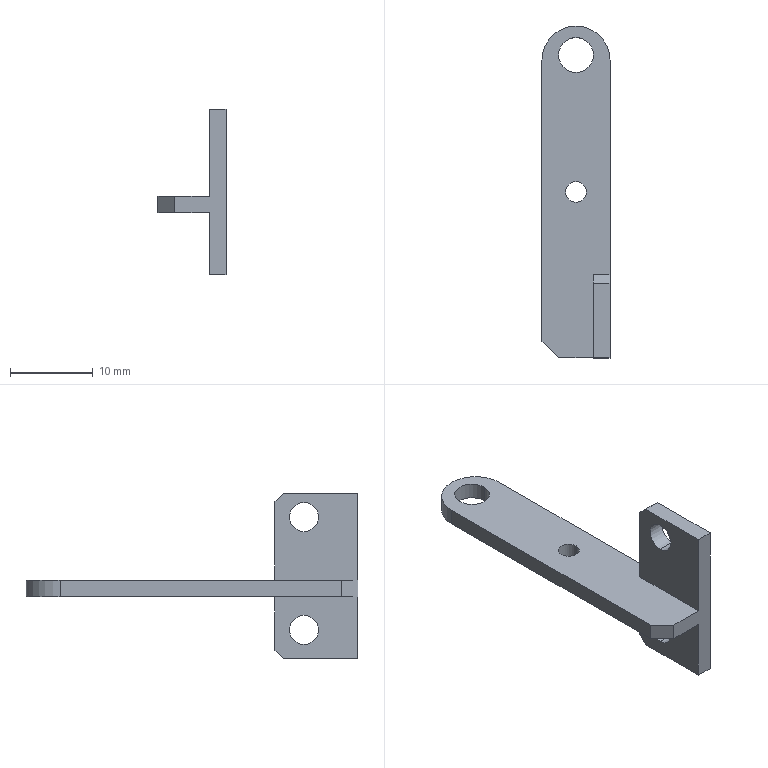Part | STEP file | 11-FG-B07711 | 1 solid | 24 faces | box 8.2 x 40 x 20 mm | volume 919.559 mm3 | plane 14 | cylinder 10 | commonest cylinder face diameters 3.5 x4 2.5 x2 4.2 x2 8.2 x2
STEP:
#1=CARTESIAN_POINT('',(-1.25,0.,0.));
#2=VERTEX_POINT('',#1);
#3=CARTESIAN_POINT('',(1.25,0.,0.));
#4=VERTEX_POINT('',#3);
#5=CARTESIAN_POINT('',(0.,0.,0.));
#6=DIRECTION('',(0.,0.,1.));
#7=DIRECTION('',(1.,0.,0.));
#8=AXIS2_PLACEMENT_3D('',#5,#6,#7);
#9=CIRCLE('',#8,1.25);
#10=EDGE_CURVE('',#2,#4,#9,.T.);
#11=ORIENTED_EDGE('',*,*,#10,.F.);
#12=CARTESIAN_POINT('',(-1.25,0.,2.));
#13=VERTEX_POINT('',#12);
#14=CARTESIAN_POINT('',(-1.25,0.,2.));
#15=DIRECTION('',(0.,0.,1.));
#16=VECTOR('',#15,1000.);
#17=LINE('',#14,#16);
#18=EDGE_CURVE('',#2,#13,#17,.T.);
#19=ORIENTED_EDGE('',*,*,#18,.T.);
#20=CARTESIAN_POINT('',(1.25,0.,2.));
#21=VERTEX_POINT('',#20);
#22=CARTESIAN_POINT('',(0.,0.,2.));
#23=DIRECTION('',(0.,0.,1.));
#24=DIRECTION('',(1.,0.,0.));
#25=AXIS2_PLACEMENT_3D('',#22,#23,#24);
#26=CIRCLE('',#25,1.25);
#27=EDGE_CURVE('',#13,#21,#26,.T.);
#28=ORIENTED_EDGE('',*,*,#27,.T.);
#29=CARTESIAN_POINT('',(1.25,0.,2.));
#30=DIRECTION('',(0.,0.,1.));
#31=VECTOR('',#30,1000.);
#32=LINE('',#29,#31);
#33=EDGE_CURVE('',#4,#21,#32,.T.);
#34=ORIENTED_EDGE('',*,*,#33,.F.);
#35=EDGE_LOOP('',(#11,#19,#28,#34));
#36=FACE_OUTER_BOUND('',#35,.T.);
#37=CARTESIAN_POINT('',(0.,0.,2.));
#38=DIRECTION('',(0.,0.,1.));
#39=DIRECTION('',(1.,0.,0.));
#40=AXIS2_PLACEMENT_3D('',#37,#38,#39);
#41=CYLINDRICAL_SURFACE('',#40,1.25);
#42=ADVANCED_FACE('',(#36),#41,.F.);
#43=CARTESIAN_POINT('',(4.1,-13.5,-5.75));
#44=VERTEX_POINT('',#43);
#45=CARTESIAN_POINT('',(4.1,-13.5,-2.25));
#46=VERTEX_POINT('',#45);
#47=CARTESIAN_POINT('',(4.1,-13.5,-4.));
#48=DIRECTION('',(-1.,0.,0.));
#49=DIRECTION('',(0.,-1.,0.));
#50=AXIS2_PLACEMENT_3D('',#47,#48,#49);
#51=CIRCLE('',#50,1.75);
#52=EDGE_CURVE('',#44,#46,#51,.T.);
#53=ORIENTED_EDGE('',*,*,#52,.F.);
#54=CARTESIAN_POINT('',(2.1,-13.5,-5.75));
#55=VERTEX_POINT('',#54);
#56=CARTESIAN_POINT('',(9.6,-13.5,-5.75));
#57=DIRECTION('',(-1.,0.,0.));
#58=VECTOR('',#57,1000.);
#59=LINE('',#56,#58);
#60=EDGE_CURVE('',#44,#55,#59,.T.);
#61=ORIENTED_EDGE('',*,*,#60,.T.);
#62=CARTESIAN_POINT('',(2.1,-13.5,-2.25));
#63=VERTEX_POINT('',#62);
#64=CARTESIAN_POINT('',(2.1,-13.5,-4.));
#65=DIRECTION('',(-1.,0.,0.));
#66=DIRECTION('',(0.,0.,1.));
#67=AXIS2_PLACEMENT_3D('',#64,#65,#66);
#68=CIRCLE('',#67,1.75);
#69=EDGE_CURVE('',#55,#63,#68,.T.);
#70=ORIENTED_EDGE('',*,*,#69,.T.);
#71=CARTESIAN_POINT('',(9.6,-13.5,-2.25));
#72=DIRECTION('',(-1.,0.,0.));
#73=VECTOR('',#72,1000.);
#74=LINE('',#71,#73);
#75=EDGE_CURVE('',#46,#63,#74,.T.);
#76=ORIENTED_EDGE('',*,*,#75,.F.);
#77=EDGE_LOOP('',(#53,#61,#70,#76));
#78=FACE_OUTER_BOUND('',#77,.T.);
#79=CARTESIAN_POINT('',(9.6,-13.5,-4.));
#80=DIRECTION('',(-1.,0.,0.));
#81=DIRECTION('',(0.,0.,1.));
#82=AXIS2_PLACEMENT_3D('',#79,#80,#81);
#83=CYLINDRICAL_SURFACE('',#82,1.75);
#84=ADVANCED_FACE('',(#78),#83,.F.);
#85=CARTESIAN_POINT('',(4.1,-13.5,7.85));
#86=VERTEX_POINT('',#85);
#87=CARTESIAN_POINT('',(4.1,-13.5,11.35));
#88=VERTEX_POINT('',#87);
#89=CARTESIAN_POINT('',(4.1,-13.5,9.6));
#90=DIRECTION('',(-1.,0.,0.));
#91=DIRECTION('',(0.,-1.,0.));
#92=AXIS2_PLACEMENT_3D('',#89,#90,#91);
#93=CIRCLE('',#92,1.75);
#94=EDGE_CURVE('',#86,#88,#93,.T.);
#95=ORIENTED_EDGE('',*,*,#94,.F.);
#96=CARTESIAN_POINT('',(2.1,-13.5,7.85));
#97=VERTEX_POINT('',#96);
#98=CARTESIAN_POINT('',(9.6,-13.5,7.85));
#99=DIRECTION('',(-1.,0.,0.));
#100=VECTOR('',#99,1000.);
#101=LINE('',#98,#100);
#102=EDGE_CURVE('',#86,#97,#101,.T.);
#103=ORIENTED_EDGE('',*,*,#102,.T.);
#104=CARTESIAN_POINT('',(2.1,-13.5,11.35));
#105=VERTEX_POINT('',#104);
#106=CARTESIAN_POINT('',(2.1,-13.5,9.6));
#107=DIRECTION('',(-1.,0.,0.));
#108=DIRECTION('',(0.,0.,1.));
#109=AXIS2_PLACEMENT_3D('',#106,#107,#108);
#110=CIRCLE('',#109,1.75);
#111=EDGE_CURVE('',#97,#105,#110,.T.);
#112=ORIENTED_EDGE('',*,*,#111,.T.);
#113=CARTESIAN_POINT('',(9.6,-13.5,11.35));
#114=DIRECTION('',(-1.,0.,0.));
#115=VECTOR('',#114,1000.);
#116=LINE('',#113,#115);
#117=EDGE_CURVE('',#88,#105,#116,.T.);
#118=ORIENTED_EDGE('',*,*,#117,.F.);
#119=EDGE_LOOP('',(#95,#103,#112,#118));
#120=FACE_OUTER_BOUND('',#119,.T.);
#121=CARTESIAN_POINT('',(9.6,-13.5,9.6));
#122=DIRECTION('',(-1.,0.,0.));
#123=DIRECTION('',(0.,0.,1.));
#124=AXIS2_PLACEMENT_3D('',#121,#122,#123);
#125=CYLINDRICAL_SURFACE('',#124,1.75);
#126=ADVANCED_FACE('',(#120),#125,.F.);
#127=CARTESIAN_POINT('',(-2.1,16.5,0.));
#128=VERTEX_POINT('',#127);
#129=CARTESIAN_POINT('',(2.1,16.5,0.));
#130=VERTEX_POINT('',#129);
#131=CARTESIAN_POINT('',(0.,16.5,0.));
#132=DIRECTION('',(0.,0.,1.));
#133=DIRECTION('',(1.,0.,0.));
#134=AXIS2_PLACEMENT_3D('',#131,#132,#133);
#135=CIRCLE('',#134,2.1);
#136=EDGE_CURVE('',#128,#130,#135,.T.);
#137=ORIENTED_EDGE('',*,*,#136,.F.);
#138=CARTESIAN_POINT('',(-2.1,16.5,2.));
#139=VERTEX_POINT('',#138);
#140=CARTESIAN_POINT('',(-2.1,16.5,0.));
#141=DIRECTION('',(0.,0.,1.));
#142=VECTOR('',#141,1000.);
#143=LINE('',#140,#142);
#144=EDGE_CURVE('',#128,#139,#143,.T.);
#145=ORIENTED_EDGE('',*,*,#144,.T.);
#146=CARTESIAN_POINT('',(2.1,16.5,2.));
#147=VERTEX_POINT('',#146);
#148=CARTESIAN_POINT('',(0.,16.5,2.));
#149=DIRECTION('',(0.,0.,1.));
#150=DIRECTION('',(1.,0.,0.));
#151=AXIS2_PLACEMENT_3D('',#148,#149,#150);
#152=CIRCLE('',#151,2.1);
#153=EDGE_CURVE('',#139,#147,#152,.T.);
#154=ORIENTED_EDGE('',*,*,#153,.T.);
#155=CARTESIAN_POINT('',(2.1,16.5,0.));
#156=DIRECTION('',(0.,0.,1.));
#157=VECTOR('',#156,1000.);
#158=LINE('',#155,#157);
#159=EDGE_CURVE('',#130,#147,#158,.T.);
#160=ORIENTED_EDGE('',*,*,#159,.F.);
#161=EDGE_LOOP('',(#137,#145,#154,#160));
#162=FACE_OUTER_BOUND('',#161,.T.);
#163=CARTESIAN_POINT('',(0.,16.5,0.));
#164=DIRECTION('',(0.,0.,1.));
#165=DIRECTION('',(1.,0.,0.));
#166=AXIS2_PLACEMENT_3D('',#163,#164,#165);
#167=CYLINDRICAL_SURFACE('',#166,2.1);
#168=ADVANCED_FACE('',(#162),#167,.F.);
#169=CARTESIAN_POINT('',(0.,0.,0.));
#170=DIRECTION('',(0.,0.,1.));
#171=DIRECTION('',(1.,0.,0.));
#172=AXIS2_PLACEMENT_3D('',#169,#170,#171);
#173=CIRCLE('',#172,1.25);
#174=EDGE_CURVE('',#4,#2,#173,.T.);
#175=ORIENTED_EDGE('',*,*,#174,.T.);
#176=ORIENTED_EDGE('',*,*,#10,.T.);
#177=EDGE_LOOP('',(#175,#176));
#178=FACE_BOUND('',#177,.T.);
#179=CARTESIAN_POINT('',(0.,16.5,0.));
#180=DIRECTION('',(0.,0.,1.));
#181=DIRECTION('',(1.,0.,0.));
#182=AXIS2_PLACEMENT_3D('',#179,#180,#181);
#183=CIRCLE('',#182,2.1);
#184=EDGE_CURVE('',#130,#128,#183,.T.);
#185=ORIENTED_EDGE('',*,*,#184,.T.);
#186=ORIENTED_EDGE('',*,*,#136,.T.);
#187=EDGE_LOOP('',(#185,#186));
#188=FACE_BOUND('',#187,.T.);
#189=CARTESIAN_POINT('',(-2.1,-20.,0.));
#190=VERTEX_POINT('',#189);
#191=CARTESIAN_POINT('',(2.1,-20.,0.));
#192=VERTEX_POINT('',#191);
#193=CARTESIAN_POINT('',(-14.1,-20.,0.));
#194=DIRECTION('',(1.,0.,0.));
#195=VECTOR('',#194,1000.);
#196=LINE('',#193,#195);
#197=EDGE_CURVE('',#190,#192,#196,.T.);
#198=ORIENTED_EDGE('',*,*,#197,.F.);
#199=CARTESIAN_POINT('',(-4.1,-18.,0.));
#200=VERTEX_POINT('',#199);
#201=CARTESIAN_POINT('',(-4.1,-18.,0.));
#202=DIRECTION('',(-0.7071,0.7071,0.));
#203=VECTOR('',#202,1000.);
#204=LINE('',#201,#203);
#205=EDGE_CURVE('',#190,#200,#204,.T.);
#206=ORIENTED_EDGE('',*,*,#205,.T.);
#207=CARTESIAN_POINT('',(-4.1,15.9,0.));
#208=VERTEX_POINT('',#207);
#209=CARTESIAN_POINT('',(-4.1,20.,0.));
#210=DIRECTION('',(0.,1.,0.));
#211=VECTOR('',#210,1000.);
#212=LINE('',#209,#211);
#213=EDGE_CURVE('',#200,#208,#212,.T.);
#214=ORIENTED_EDGE('',*,*,#213,.T.);
#215=CARTESIAN_POINT('',(0.,20.,0.));
#216=VERTEX_POINT('',#215);
#217=CARTESIAN_POINT('',(0.,15.9,0.));
#218=DIRECTION('',(0.,0.,-1.));
#219=DIRECTION('',(1.,0.,0.));
#220=AXIS2_PLACEMENT_3D('',#217,#218,#219);
#221=CIRCLE('',#220,4.1);
#222=EDGE_CURVE('',#208,#216,#221,.T.);
#223=ORIENTED_EDGE('',*,*,#222,.T.);
#224=CARTESIAN_POINT('',(4.1,15.9,0.));
#225=VERTEX_POINT('',#224);
#226=CARTESIAN_POINT('',(0.,15.9,0.));
#227=DIRECTION('',(0.,0.,-1.));
#228=DIRECTION('',(1.,0.,0.));
#229=AXIS2_PLACEMENT_3D('',#226,#227,#228);
#230=CIRCLE('',#229,4.1);
#231=EDGE_CURVE('',#216,#225,#230,.T.);
#232=ORIENTED_EDGE('',*,*,#231,.T.);
#233=CARTESIAN_POINT('',(4.1,-10.,0.));
#234=VERTEX_POINT('',#233);
#235=CARTESIAN_POINT('',(4.1,20.,0.));
#236=DIRECTION('',(0.,-1.,0.));
#237=VECTOR('',#236,1000.);
#238=LINE('',#235,#237);
#239=EDGE_CURVE('',#225,#234,#238,.T.);
#240=ORIENTED_EDGE('',*,*,#239,.T.);
#241=CARTESIAN_POINT('',(2.1,-10.,0.));
#242=VERTEX_POINT('',#241);
#243=CARTESIAN_POINT('',(2.1,-10.,0.));
#244=DIRECTION('',(1.,0.,0.));
#245=VECTOR('',#244,1000.);
#246=LINE('',#243,#245);
#247=EDGE_CURVE('',#242,#234,#246,.T.);
#248=ORIENTED_EDGE('',*,*,#247,.F.);
#249=CARTESIAN_POINT('',(2.1,-10.,0.));
#250=DIRECTION('',(0.,1.,0.));
#251=VECTOR('',#250,1000.);
#252=LINE('',#249,#251);
#253=EDGE_CURVE('',#192,#242,#252,.T.);
#254=ORIENTED_EDGE('',*,*,#253,.F.);
#255=EDGE_LOOP('',(#198,#206,#214,#223,#232,#240,#248,#254));
#256=FACE_OUTER_BOUND('',#255,.T.);
#257=CARTESIAN_POINT('',(0.,0.,0.));
#258=DIRECTION('',(0.,0.,1.));
#259=DIRECTION('',(1.,0.,0.));
#260=AXIS2_PLACEMENT_3D('',#257,#258,#259);
#261=PLANE('',#260);
#262=ADVANCED_FACE('',(#178,#188,#256),#261,.F.);
#263=CARTESIAN_POINT('',(-2.1,-20.,2.));
#264=VERTEX_POINT('',#263);
#265=CARTESIAN_POINT('',(2.1,-20.,2.));
#266=VERTEX_POINT('',#265);
#267=CARTESIAN_POINT('',(-14.1,-20.,2.));
#268=DIRECTION('',(1.,0.,0.));
#269=VECTOR('',#268,1000.);
#270=LINE('',#267,#269);
#271=EDGE_CURVE('',#264,#266,#270,.T.);
#272=ORIENTED_EDGE('',*,*,#271,.F.);
#273=CARTESIAN_POINT('',(-2.1,-20.,2.));
#274=DIRECTION('',(0.,0.,-1.));
#275=VECTOR('',#274,1000.);
#276=LINE('',#273,#275);
#277=EDGE_CURVE('',#264,#190,#276,.T.);
#278=ORIENTED_EDGE('',*,*,#277,.T.);
#279=ORIENTED_EDGE('',*,*,#197,.T.);
#280=CARTESIAN_POINT('',(2.1,-20.,-7.5));
#281=VERTEX_POINT('',#280);
#282=CARTESIAN_POINT('',(2.1,-20.,-7.5));
#283=DIRECTION('',(0.,0.,1.));
#284=VECTOR('',#283,1000.);
#285=LINE('',#282,#284);
#286=EDGE_CURVE('',#281,#192,#285,.T.);
#287=ORIENTED_EDGE('',*,*,#286,.F.);
#288=CARTESIAN_POINT('',(4.1,-20.,-7.5));
#289=VERTEX_POINT('',#288);
#290=CARTESIAN_POINT('',(2.1,-20.,-7.5));
#291=DIRECTION('',(-1.,0.,0.));
#292=VECTOR('',#291,1000.);
#293=LINE('',#290,#292);
#294=EDGE_CURVE('',#289,#281,#293,.T.);
#295=ORIENTED_EDGE('',*,*,#294,.F.);
#296=CARTESIAN_POINT('',(4.1,-20.,12.5));
#297=VERTEX_POINT('',#296);
#298=CARTESIAN_POINT('',(4.1,-20.,-22.));
#299=DIRECTION('',(0.,0.,1.));
#300=VECTOR('',#299,1000.);
#301=LINE('',#298,#300);
#302=EDGE_CURVE('',#289,#297,#301,.T.);
#303=ORIENTED_EDGE('',*,*,#302,.T.);
#304=CARTESIAN_POINT('',(2.1,-20.,12.5));
#305=VERTEX_POINT('',#304);
#306=CARTESIAN_POINT('',(4.1,-20.,12.5));
#307=DIRECTION('',(1.,0.,0.));
#308=VECTOR('',#307,1000.);
#309=LINE('',#306,#308);
#310=EDGE_CURVE('',#305,#297,#309,.T.);
#311=ORIENTED_EDGE('',*,*,#310,.F.);
#312=CARTESIAN_POINT('',(2.1,-20.,12.5));
#313=DIRECTION('',(0.,0.,-1.));
#314=VECTOR('',#313,1000.);
#315=LINE('',#312,#314);
#316=EDGE_CURVE('',#305,#266,#315,.T.);
#317=ORIENTED_EDGE('',*,*,#316,.T.);
#318=EDGE_LOOP('',(#272,#278,#279,#287,#295,#303,#311,#317));
#319=FACE_OUTER_BOUND('',#318,.T.);
#320=CARTESIAN_POINT('',(-14.1,-20.,2.));
#321=DIRECTION('',(0.,1.,0.));
#322=DIRECTION('',(0.,0.,1.));
#323=AXIS2_PLACEMENT_3D('',#320,#321,#322);
#324=PLANE('',#323);
#325=ADVANCED_FACE('',(#319),#324,.F.);
#326=CARTESIAN_POINT('',(0.,0.,2.));
#327=DIRECTION('',(0.,0.,1.));
#328=DIRECTION('',(1.,0.,0.));
#329=AXIS2_PLACEMENT_3D('',#326,#327,#328);
#330=CIRCLE('',#329,1.25);
#331=EDGE_CURVE('',#21,#13,#330,.T.);
#332=ORIENTED_EDGE('',*,*,#331,.F.);
#333=ORIENTED_EDGE('',*,*,#27,.F.);
#334=EDGE_LOOP('',(#332,#333));
#335=FACE_BOUND('',#334,.T.);
#336=CARTESIAN_POINT('',(-4.1,-18.,2.));
#337=VERTEX_POINT('',#336);
#338=CARTESIAN_POINT('',(-4.1,15.9,2.));
#339=VERTEX_POINT('',#338);
#340=CARTESIAN_POINT('',(-4.1,20.,2.));
#341=DIRECTION('',(0.,1.,0.));
#342=VECTOR('',#341,1000.);
#343=LINE('',#340,#342);
#344=EDGE_CURVE('',#337,#339,#343,.T.);
#345=ORIENTED_EDGE('',*,*,#344,.F.);
#346=CARTESIAN_POINT('',(-11.05,-11.05,2.));
#347=DIRECTION('',(0.7071,-0.7071,0.));
#348=VECTOR('',#347,1000.);
#349=LINE('',#346,#348);
#350=EDGE_CURVE('',#337,#264,#349,.T.);
#351=ORIENTED_EDGE('',*,*,#350,.T.);
#352=ORIENTED_EDGE('',*,*,#271,.T.);
#353=CARTESIAN_POINT('',(2.1,-10.,2.));
#354=VERTEX_POINT('',#353);
#355=CARTESIAN_POINT('',(2.1,-20.,2.));
#356=DIRECTION('',(0.,-1.,0.));
#357=VECTOR('',#356,1000.);
#358=LINE('',#355,#357);
#359=EDGE_CURVE('',#354,#266,#358,.T.);
#360=ORIENTED_EDGE('',*,*,#359,.F.);
#361=CARTESIAN_POINT('',(4.1,-10.,2.));
#362=VERTEX_POINT('',#361);
#363=CARTESIAN_POINT('',(4.1,-10.,2.));
#364=DIRECTION('',(-1.,0.,0.));
#365=VECTOR('',#364,1000.);
#366=LINE('',#363,#365);
#367=EDGE_CURVE('',#362,#354,#366,.T.);
#368=ORIENTED_EDGE('',*,*,#367,.F.);
#369=CARTESIAN_POINT('',(4.1,15.9,2.));
#370=VERTEX_POINT('',#369);
#371=CARTESIAN_POINT('',(4.1,20.,2.));
#372=DIRECTION('',(0.,-1.,0.));
#373=VECTOR('',#372,1000.);
#374=LINE('',#371,#373);
#375=EDGE_CURVE('',#370,#362,#374,.T.);
#376=ORIENTED_EDGE('',*,*,#375,.F.);
#377=CARTESIAN_POINT('',(0.,20.,2.));
#378=VERTEX_POINT('',#377);
#379=CARTESIAN_POINT('',(0.,15.9,2.));
#380=DIRECTION('',(0.,0.,1.));
#381=DIRECTION('',(1.,0.,0.));
#382=AXIS2_PLACEMENT_3D('',#379,#380,#381);
#383=CIRCLE('',#382,4.1);
#384=EDGE_CURVE('',#370,#378,#383,.T.);
#385=ORIENTED_EDGE('',*,*,#384,.T.);
#386=CARTESIAN_POINT('',(0.,15.9,2.));
#387=DIRECTION('',(0.,0.,1.));
#388=DIRECTION('',(1.,0.,0.));
#389=AXIS2_PLACEMENT_3D('',#386,#387,#388);
#390=CIRCLE('',#389,4.1);
#391=EDGE_CURVE('',#378,#339,#390,.T.);
#392=ORIENTED_EDGE('',*,*,#391,.T.);
#393=EDGE_LOOP('',(#345,#351,#352,#360,#368,#376,#385,#392));
#394=FACE_OUTER_BOUND('',#393,.T.);
#395=CARTESIAN_POINT('',(0.,16.5,2.));
#396=DIRECTION('',(0.,0.,1.));
#397=DIRECTION('',(1.,0.,0.));
#398=AXIS2_PLACEMENT_3D('',#395,#396,#397);
#399=CIRCLE('',#398,2.1);
#400=EDGE_CURVE('',#147,#139,#399,.T.);
#401=ORIENTED_EDGE('',*,*,#400,.F.);
#402=ORIENTED_EDGE('',*,*,#153,.F.);
#403=EDGE_LOOP('',(#401,#402));
#404=FACE_BOUND('',#403,.T.);
#405=CARTESIAN_POINT('',(0.,0.,2.));
#406=DIRECTION('',(0.,0.,1.));
#407=DIRECTION('',(1.,0.,0.));
#408=AXIS2_PLACEMENT_3D('',#405,#406,#407);
#409=PLANE('',#408);
#410=ADVANCED_FACE('',(#335,#394,#404),#409,.T.);
#411=ORIENTED_EDGE('',*,*,#213,.F.);
#412=CARTESIAN_POINT('',(-4.1,-18.,0.));
#413=DIRECTION('',(0.,0.,1.));
#414=VECTOR('',#413,1000.);
#415=LINE('',#412,#414);
#416=EDGE_CURVE('',#200,#337,#415,.T.);
#417=ORIENTED_EDGE('',*,*,#416,.T.);
#418=ORIENTED_EDGE('',*,*,#344,.T.);
#419=CARTESIAN_POINT('',(-4.1,15.9,0.));
#420=DIRECTION('',(0.,0.,-1.));
#421=VECTOR('',#420,1000.);
#422=LINE('',#419,#421);
#423=EDGE_CURVE('',#339,#208,#422,.T.);
#424=ORIENTED_EDGE('',*,*,#423,.T.);
#425=EDGE_LOOP('',(#411,#417,#418,#424));
#426=FACE_OUTER_BOUND('',#425,.T.);
#427=CARTESIAN_POINT('',(-4.1,20.,0.));
#428=DIRECTION('',(1.,0.,0.));
#429=DIRECTION('',(0.,1.,0.));
#430=AXIS2_PLACEMENT_3D('',#427,#428,#429);
#431=PLANE('',#430);
#432=ADVANCED_FACE('',(#426),#431,.F.);
#433=CARTESIAN_POINT('',(4.1,-13.5,-4.));
#434=DIRECTION('',(-1.,0.,0.));
#435=DIRECTION('',(0.,-1.,0.));
#436=AXIS2_PLACEMENT_3D('',#433,#434,#435);
#437=CIRCLE('',#436,1.75);
#438=EDGE_CURVE('',#46,#44,#437,.T.);
#439=ORIENTED_EDGE('',*,*,#438,.T.);
#440=ORIENTED_EDGE('',*,*,#52,.T.);
#441=EDGE_LOOP('',(#439,#440));
#442=FACE_BOUND('',#441,.T.);
#443=CARTESIAN_POINT('',(4.1,-13.5,9.6));
#444=DIRECTION('',(-1.,0.,0.));
#445=DIRECTION('',(0.,-1.,0.));
#446=AXIS2_PLACEMENT_3D('',#443,#444,#445);
#447=CIRCLE('',#446,1.75);
#448=EDGE_CURVE('',#88,#86,#447,.T.);
#449=ORIENTED_EDGE('',*,*,#448,.T.);
#450=ORIENTED_EDGE('',*,*,#94,.T.);
#451=EDGE_LOOP('',(#449,#450));
#452=FACE_BOUND('',#451,.T.);
#453=CARTESIAN_POINT('',(4.1,-11.,-7.5));
#454=VERTEX_POINT('',#453);
#455=CARTESIAN_POINT('',(4.1,-10.,-7.5));
#456=DIRECTION('',(0.,-1.,0.));
#457=VECTOR('',#456,1000.);
#458=LINE('',#455,#457);
#459=EDGE_CURVE('',#454,#289,#458,.T.);
#460=ORIENTED_EDGE('',*,*,#459,.F.);
#461=CARTESIAN_POINT('',(4.1,-10.,-6.5));
#462=VERTEX_POINT('',#461);
#463=CARTESIAN_POINT('',(4.1,-11.,-7.5));
#464=DIRECTION('',(0.,0.7071,0.7071));
#465=VECTOR('',#464,1000.);
#466=LINE('',#463,#465);
#467=EDGE_CURVE('',#454,#462,#466,.T.);
#468=ORIENTED_EDGE('',*,*,#467,.T.);
#469=CARTESIAN_POINT('',(4.1,-10.,-7.5));
#470=DIRECTION('',(0.,0.,1.));
#471=VECTOR('',#470,1000.);
#472=LINE('',#469,#471);
#473=EDGE_CURVE('',#462,#234,#472,.T.);
#474=ORIENTED_EDGE('',*,*,#473,.T.);
#475=ORIENTED_EDGE('',*,*,#239,.F.);
#476=CARTESIAN_POINT('',(4.1,15.9,0.));
#477=DIRECTION('',(0.,0.,1.));
#478=VECTOR('',#477,1000.);
#479=LINE('',#476,#478);
#480=EDGE_CURVE('',#225,#370,#479,.T.);
#481=ORIENTED_EDGE('',*,*,#480,.T.);
#482=ORIENTED_EDGE('',*,*,#375,.T.);
#483=CARTESIAN_POINT('',(4.1,-10.,11.5));
#484=VERTEX_POINT('',#483);
#485=CARTESIAN_POINT('',(4.1,-10.,12.5));
#486=DIRECTION('',(0.,0.,-1.));
#487=VECTOR('',#486,1000.);
#488=LINE('',#485,#487);
#489=EDGE_CURVE('',#484,#362,#488,.T.);
#490=ORIENTED_EDGE('',*,*,#489,.F.);
#491=CARTESIAN_POINT('',(4.1,-11.,12.5));
#492=VERTEX_POINT('',#491);
#493=CARTESIAN_POINT('',(4.1,-11.,12.5));
#494=DIRECTION('',(0.,-0.7071,0.7071));
#495=VECTOR('',#494,1000.);
#496=LINE('',#493,#495);
#497=EDGE_CURVE('',#484,#492,#496,.T.);
#498=ORIENTED_EDGE('',*,*,#497,.T.);
#499=CARTESIAN_POINT('',(4.1,-20.,12.5));
#500=DIRECTION('',(0.,1.,0.));
#501=VECTOR('',#500,1000.);
#502=LINE('',#499,#501);
#503=EDGE_CURVE('',#297,#492,#502,.T.);
#504=ORIENTED_EDGE('',*,*,#503,.F.);
#505=ORIENTED_EDGE('',*,*,#302,.F.);
#506=EDGE_LOOP('',(#460,#468,#474,#475,#481,#482,#490,#498,#504,#505));
#507=FACE_OUTER_BOUND('',#506,.T.);
#508=CARTESIAN_POINT('',(4.1,20.,0.));
#509=DIRECTION('',(-1.,0.,0.));
#510=DIRECTION('',(0.,-1.,0.));
#511=AXIS2_PLACEMENT_3D('',#508,#509,#510);
#512=PLANE('',#511);
#513=ADVANCED_FACE('',(#442,#452,#507),#512,.F.);
#514=ORIENTED_EDGE('',*,*,#144,.F.);
#515=ORIENTED_EDGE('',*,*,#184,.F.);
#516=ORIENTED_EDGE('',*,*,#159,.T.);
#517=ORIENTED_EDGE('',*,*,#400,.T.);
#518=EDGE_LOOP('',(#514,#515,#516,#517));
#519=FACE_OUTER_BOUND('',#518,.T.);
#520=CARTESIAN_POINT('',(0.,16.5,0.));
#521=DIRECTION('',(0.,0.,1.));
#522=DIRECTION('',(1.,0.,0.));
#523=AXIS2_PLACEMENT_3D('',#520,#521,#522);
#524=CYLINDRICAL_SURFACE('',#523,2.1);
#525=ADVANCED_FACE('',(#519),#524,.F.);
#526=CARTESIAN_POINT('',(0.,20.,2.));
#527=DIRECTION('',(0.,0.,1.));
#528=VECTOR('',#527,1000.);
#529=LINE('',#526,#528);
#530=EDGE_CURVE('',#216,#378,#529,.T.);
#531=ORIENTED_EDGE('',*,*,#530,.F.);
#532=ORIENTED_EDGE('',*,*,#222,.F.);
#533=ORIENTED_EDGE('',*,*,#423,.F.);
#534=ORIENTED_EDGE('',*,*,#391,.F.);
#535=EDGE_LOOP('',(#531,#532,#533,#534));
#536=FACE_OUTER_BOUND('',#535,.T.);
#537=CARTESIAN_POINT('',(0.,15.9,2.));
#538=DIRECTION('',(0.,0.,1.));
#539=DIRECTION('',(1.,0.,0.));
#540=AXIS2_PLACEMENT_3D('',#537,#538,#539);
#541=CYLINDRICAL_SURFACE('',#540,4.1);
#542=ADVANCED_FACE('',(#536),#541,.T.);
#543=ORIENTED_EDGE('',*,*,#231,.F.);
#544=ORIENTED_EDGE('',*,*,#530,.T.);
#545=ORIENTED_EDGE('',*,*,#384,.F.);
#546=ORIENTED_EDGE('',*,*,#480,.F.);
#547=EDGE_LOOP('',(#543,#544,#545,#546));
#548=FACE_OUTER_BOUND('',#547,.T.);
#549=CARTESIAN_POINT('',(0.,15.9,0.));
#550=DIRECTION('',(0.,0.,1.));
#551=DIRECTION('',(1.,0.,0.));
#552=AXIS2_PLACEMENT_3D('',#549,#550,#551);
#553=CYLINDRICAL_SURFACE('',#552,4.1);
#554=ADVANCED_FACE('',(#548),#553,.T.);
#555=CARTESIAN_POINT('',(2.1,-10.,11.5));
#556=VERTEX_POINT('',#555);
#557=CARTESIAN_POINT('',(2.1,-10.,12.5));
#558=DIRECTION('',(0.,0.,-1.));
#559=VECTOR('',#558,1000.);
#560=LINE('',#557,#559);
#561=EDGE_CURVE('',#556,#354,#560,.T.);
#562=ORIENTED_EDGE('',*,*,#561,.F.);
#563=CARTESIAN_POINT('',(4.1,-10.,11.5));
#564=DIRECTION('',(1.,0.,0.));
#565=VECTOR('',#564,1000.);
#566=LINE('',#563,#565);
#567=EDGE_CURVE('',#556,#484,#566,.T.);
#568=ORIENTED_EDGE('',*,*,#567,.T.);
#569=ORIENTED_EDGE('',*,*,#489,.T.);
#570=ORIENTED_EDGE('',*,*,#367,.T.);
#571=EDGE_LOOP('',(#562,#568,#569,#570));
#572=FACE_OUTER_BOUND('',#571,.T.);
#573=CARTESIAN_POINT('',(4.1,-10.,12.5));
#574=DIRECTION('',(0.,-1.,0.));
#575=DIRECTION('',(1.,0.,0.));
#576=AXIS2_PLACEMENT_3D('',#573,#574,#575);
#577=PLANE('',#576);
#578=ADVANCED_FACE('',(#572),#577,.F.);
#579=CARTESIAN_POINT('',(2.1,-13.5,9.6));
#580=DIRECTION('',(-1.,0.,0.));
#581=DIRECTION('',(0.,0.,1.));
#582=AXIS2_PLACEMENT_3D('',#579,#580,#581);
#583=CIRCLE('',#582,1.75);
#584=EDGE_CURVE('',#105,#97,#583,.T.);
#585=ORIENTED_EDGE('',*,*,#584,.F.);
#586=ORIENTED_EDGE('',*,*,#111,.F.);
#587=EDGE_LOOP('',(#585,#586));
#588=FACE_BOUND('',#587,.T.);
#589=CARTESIAN_POINT('',(2.1,-11.,12.5));
#590=VERTEX_POINT('',#589);
#591=CARTESIAN_POINT('',(2.1,-20.,12.5));
#592=DIRECTION('',(0.,-1.,0.));
#593=VECTOR('',#592,1000.);
#594=LINE('',#591,#593);
#595=EDGE_CURVE('',#590,#305,#594,.T.);
#596=ORIENTED_EDGE('',*,*,#595,.F.);
#597=CARTESIAN_POINT('',(2.1,-11.,12.5));
#598=DIRECTION('',(0.,0.7071,-0.7071));
#599=VECTOR('',#598,1000.);
#600=LINE('',#597,#599);
#601=EDGE_CURVE('',#590,#556,#600,.T.);
#602=ORIENTED_EDGE('',*,*,#601,.T.);
#603=ORIENTED_EDGE('',*,*,#561,.T.);
#604=ORIENTED_EDGE('',*,*,#359,.T.);
#605=ORIENTED_EDGE('',*,*,#316,.F.);
#606=EDGE_LOOP('',(#596,#602,#603,#604,#605));
#607=FACE_OUTER_BOUND('',#606,.T.);
#608=CARTESIAN_POINT('',(2.1,-20.,12.5));
#609=DIRECTION('',(1.,0.,0.));
#610=DIRECTION('',(0.,0.,-1.));
#611=AXIS2_PLACEMENT_3D('',#608,#609,#610);
#612=PLANE('',#611);
#613=ADVANCED_FACE('',(#588,#607),#612,.F.);
#614=ORIENTED_EDGE('',*,*,#503,.T.);
#615=CARTESIAN_POINT('',(2.1,-11.,12.5));
#616=DIRECTION('',(-1.,0.,0.));
#617=VECTOR('',#616,1000.);
#618=LINE('',#615,#617);
#619=EDGE_CURVE('',#492,#590,#618,.T.);
#620=ORIENTED_EDGE('',*,*,#619,.T.);
#621=ORIENTED_EDGE('',*,*,#595,.T.);
#622=ORIENTED_EDGE('',*,*,#310,.T.);
#623=EDGE_LOOP('',(#614,#620,#621,#622));
#624=FACE_OUTER_BOUND('',#623,.T.);
#625=CARTESIAN_POINT('',(0.,0.,12.5));
#626=DIRECTION('',(0.,0.,1.));
#627=DIRECTION('',(1.,0.,0.));
#628=AXIS2_PLACEMENT_3D('',#625,#626,#627);
#629=PLANE('',#628);
#630=ADVANCED_FACE('',(#624),#629,.T.);
#631=CARTESIAN_POINT('',(2.1,-13.5,-4.));
#632=DIRECTION('',(-1.,0.,0.));
#633=DIRECTION('',(0.,0.,1.));
#634=AXIS2_PLACEMENT_3D('',#631,#632,#633);
#635=CIRCLE('',#634,1.75);
#636=EDGE_CURVE('',#63,#55,#635,.T.);
#637=ORIENTED_EDGE('',*,*,#636,.F.);
#638=ORIENTED_EDGE('',*,*,#69,.F.);
#639=EDGE_LOOP('',(#637,#638));
#640=FACE_BOUND('',#639,.T.);
#641=CARTESIAN_POINT('',(2.1,-10.,-6.5));
#642=VERTEX_POINT('',#641);
#643=CARTESIAN_POINT('',(2.1,-10.,-7.5));
#644=DIRECTION('',(0.,0.,1.));
#645=VECTOR('',#644,1000.);
#646=LINE('',#643,#645);
#647=EDGE_CURVE('',#642,#242,#646,.T.);
#648=ORIENTED_EDGE('',*,*,#647,.F.);
#649=CARTESIAN_POINT('',(2.1,-11.,-7.5));
#650=VERTEX_POINT('',#649);
#651=CARTESIAN_POINT('',(2.1,-11.,-7.5));
#652=DIRECTION('',(0.,-0.7071,-0.7071));
#653=VECTOR('',#652,1000.);
#654=LINE('',#651,#653);
#655=EDGE_CURVE('',#642,#650,#654,.T.);
#656=ORIENTED_EDGE('',*,*,#655,.T.);
#657=CARTESIAN_POINT('',(2.1,-10.,-7.5));
#658=DIRECTION('',(0.,1.,0.));
#659=VECTOR('',#658,1000.);
#660=LINE('',#657,#659);
#661=EDGE_CURVE('',#281,#650,#660,.T.);
#662=ORIENTED_EDGE('',*,*,#661,.F.);
#663=ORIENTED_EDGE('',*,*,#286,.T.);
#664=ORIENTED_EDGE('',*,*,#253,.T.);
#665=EDGE_LOOP('',(#648,#656,#662,#663,#664));
#666=FACE_OUTER_BOUND('',#665,.T.);
#667=CARTESIAN_POINT('',(2.1,-10.,-7.5));
#668=DIRECTION('',(1.,0.,0.));
#669=DIRECTION('',(0.,0.,-1.));
#670=AXIS2_PLACEMENT_3D('',#667,#668,#669);
#671=PLANE('',#670);
#672=ADVANCED_FACE('',(#640,#666),#671,.F.);
#673=ORIENTED_EDGE('',*,*,#473,.F.);
#674=CARTESIAN_POINT('',(2.1,-10.,-6.5));
#675=DIRECTION('',(-1.,0.,0.));
#676=VECTOR('',#675,1000.);
#677=LINE('',#674,#676);
#678=EDGE_CURVE('',#462,#642,#677,.T.);
#679=ORIENTED_EDGE('',*,*,#678,.T.);
#680=ORIENTED_EDGE('',*,*,#647,.T.);
#681=ORIENTED_EDGE('',*,*,#247,.T.);
#682=EDGE_LOOP('',(#673,#679,#680,#681));
#683=FACE_OUTER_BOUND('',#682,.T.);
#684=CARTESIAN_POINT('',(2.1,-10.,-7.5));
#685=DIRECTION('',(0.,-1.,0.));
#686=DIRECTION('',(0.,0.,-1.));
#687=AXIS2_PLACEMENT_3D('',#684,#685,#686);
#688=PLANE('',#687);
#689=ADVANCED_FACE('',(#683),#688,.F.);
#690=ORIENTED_EDGE('',*,*,#661,.T.);
#691=CARTESIAN_POINT('',(0.,-11.,-7.5));
#692=DIRECTION('',(1.,0.,0.));
#693=VECTOR('',#692,1000.);
#694=LINE('',#691,#693);
#695=EDGE_CURVE('',#650,#454,#694,.T.);
#696=ORIENTED_EDGE('',*,*,#695,.T.);
#697=ORIENTED_EDGE('',*,*,#459,.T.);
#698=ORIENTED_EDGE('',*,*,#294,.T.);
#699=EDGE_LOOP('',(#690,#696,#697,#698));
#700=FACE_OUTER_BOUND('',#699,.T.);
#701=CARTESIAN_POINT('',(0.,0.,-7.5));
#702=DIRECTION('',(0.,0.,1.));
#703=DIRECTION('',(1.,0.,0.));
#704=AXIS2_PLACEMENT_3D('',#701,#702,#703);
#705=PLANE('',#704);
#706=ADVANCED_FACE('',(#700),#705,.F.);
#707=ORIENTED_EDGE('',*,*,#102,.F.);
#708=ORIENTED_EDGE('',*,*,#448,.F.);
#709=ORIENTED_EDGE('',*,*,#117,.T.);
#710=ORIENTED_EDGE('',*,*,#584,.T.);
#711=EDGE_LOOP('',(#707,#708,#709,#710));
#712=FACE_OUTER_BOUND('',#711,.T.);
#713=CARTESIAN_POINT('',(9.6,-13.5,9.6));
#714=DIRECTION('',(-1.,0.,0.));
#715=DIRECTION('',(0.,0.,1.));
#716=AXIS2_PLACEMENT_3D('',#713,#714,#715);
#717=CYLINDRICAL_SURFACE('',#716,1.75);
#718=ADVANCED_FACE('',(#712),#717,.F.);
#719=ORIENTED_EDGE('',*,*,#60,.F.);
#720=ORIENTED_EDGE('',*,*,#438,.F.);
#721=ORIENTED_EDGE('',*,*,#75,.T.);
#722=ORIENTED_EDGE('',*,*,#636,.T.);
#723=EDGE_LOOP('',(#719,#720,#721,#722));
#724=FACE_OUTER_BOUND('',#723,.T.);
#725=CARTESIAN_POINT('',(9.6,-13.5,-4.));
#726=DIRECTION('',(-1.,0.,0.));
#727=DIRECTION('',(0.,0.,1.));
#728=AXIS2_PLACEMENT_3D('',#725,#726,#727);
#729=CYLINDRICAL_SURFACE('',#728,1.75);
#730=ADVANCED_FACE('',(#724),#729,.F.);
#731=ORIENTED_EDGE('',*,*,#205,.F.);
#732=ORIENTED_EDGE('',*,*,#277,.F.);
#733=ORIENTED_EDGE('',*,*,#350,.F.);
#734=ORIENTED_EDGE('',*,*,#416,.F.);
#735=EDGE_LOOP('',(#731,#732,#733,#734));
#736=FACE_OUTER_BOUND('',#735,.T.);
#737=CARTESIAN_POINT('',(-4.1,-18.,0.));
#738=DIRECTION('',(0.7071,0.7071,0.));
#739=DIRECTION('',(0.,0.,1.));
#740=AXIS2_PLACEMENT_3D('',#737,#738,#739);
#741=PLANE('',#740);
#742=ADVANCED_FACE('',(#736),#741,.F.);
#743=ORIENTED_EDGE('',*,*,#655,.F.);
#744=ORIENTED_EDGE('',*,*,#678,.F.);
#745=ORIENTED_EDGE('',*,*,#467,.F.);
#746=ORIENTED_EDGE('',*,*,#695,.F.);
#747=EDGE_LOOP('',(#743,#744,#745,#746));
#748=FACE_OUTER_BOUND('',#747,.T.);
#749=CARTESIAN_POINT('',(0.,-11.,-7.5));
#750=DIRECTION('',(0.,-0.7071,0.7071));
#751=DIRECTION('',(1.,0.,0.));
#752=AXIS2_PLACEMENT_3D('',#749,#750,#751);
#753=PLANE('',#752);
#754=ADVANCED_FACE('',(#748),#753,.F.);
#755=ORIENTED_EDGE('',*,*,#497,.F.);
#756=ORIENTED_EDGE('',*,*,#567,.F.);
#757=ORIENTED_EDGE('',*,*,#601,.F.);
#758=ORIENTED_EDGE('',*,*,#619,.F.);
#759=EDGE_LOOP('',(#755,#756,#757,#758));
#760=FACE_OUTER_BOUND('',#759,.T.);
#761=CARTESIAN_POINT('',(0.,-11.,12.5));
#762=DIRECTION('',(0.,0.7071,0.7071));
#763=DIRECTION('',(1.,0.,0.));
#764=AXIS2_PLACEMENT_3D('',#761,#762,#763);
#765=PLANE('',#764);
#766=ADVANCED_FACE('',(#760),#765,.T.);
#767=ORIENTED_EDGE('',*,*,#18,.F.);
#768=ORIENTED_EDGE('',*,*,#174,.F.);
#769=ORIENTED_EDGE('',*,*,#33,.T.);
#770=ORIENTED_EDGE('',*,*,#331,.T.);
#771=EDGE_LOOP('',(#767,#768,#769,#770));
#772=FACE_OUTER_BOUND('',#771,.T.);
#773=CARTESIAN_POINT('',(0.,0.,2.));
#774=DIRECTION('',(0.,0.,1.));
#775=DIRECTION('',(1.,0.,0.));
#776=AXIS2_PLACEMENT_3D('',#773,#774,#775);
#777=CYLINDRICAL_SURFACE('',#776,1.25);
#778=ADVANCED_FACE('',(#772),#777,.F.);
#779=CLOSED_SHELL('',(#42,#84,#126,#168,#262,#325,#410,#432,#513,#525,#542,#554,#578,#613,#630,#672,#689,#706,#718,#730,#742,#754,#766,#778));
#780=MANIFOLD_SOLID_BREP('',#779);
#781=CARTESIAN_POINT('',(0.,0.,0.));
#782=DIRECTION('',(0.,0.,1.));
#783=DIRECTION('',(1.,0.,0.));
#784=AXIS2_PLACEMENT_3D('',#781,#782,#783);
#785=(LENGTH_UNIT()NAMED_UNIT(*)SI_UNIT(.MILLI.,.METRE.));
#786=UNCERTAINTY_MEASURE_WITH_UNIT(LENGTH_MEASURE(0.00001),#785,'','');
#787=(NAMED_UNIT(*)PLANE_ANGLE_UNIT()SI_UNIT($,.RADIAN.));
#788=(NAMED_UNIT(*)SI_UNIT($,.STERADIAN.)SOLID_ANGLE_UNIT());
#789=(GEOMETRIC_REPRESENTATION_CONTEXT(3)GLOBAL_UNCERTAINTY_ASSIGNED_CONTEXT((#786))GLOBAL_UNIT_ASSIGNED_CONTEXT((#785,#787,#788))REPRESENTATION_CONTEXT('',''));
#790=ADVANCED_BREP_SHAPE_REPRESENTATION('',(#780,#784),#789);